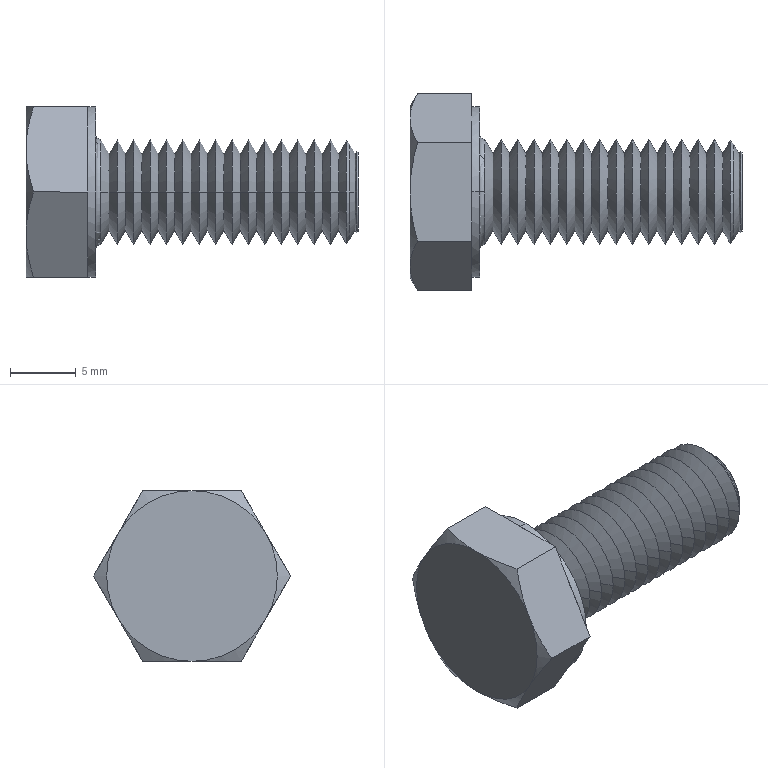Part | SolidWorks | features RevCut 4, Chamfer 1, Extrusion 1, Fillet 1, LPattern 1, Revolution 1 | 1 solid | 121 faces | box 25.3 x 15.011 x 13 mm | volume 1526 mm3 | cone 74 | cylinder 30 | plane 15 | torus 2 | commonest cylinder face diameters 8 x28 13 x2